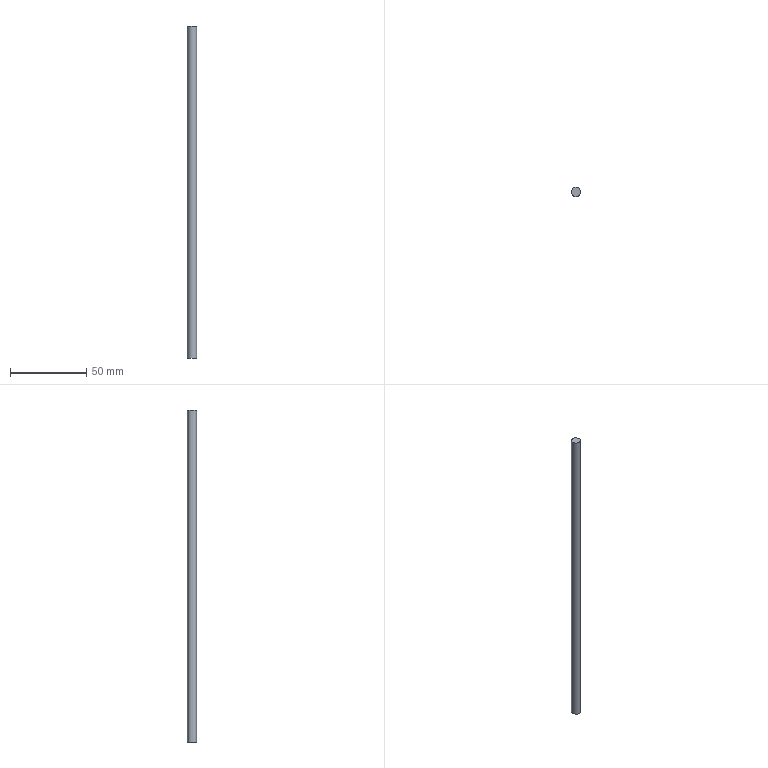Part | NX | features solid 2 | 1 solid | 3 faces | box 6 x 6 x 218 mm | volume 6164 mm3 | plane 2 | cylinder 1 | commonest cylinder face diameters 6 x1
STEP:
#1=CARTESIAN_POINT('',(157.5,-129.5,-423.));
#2=VERTEX_POINT('',#1);
#3=CARTESIAN_POINT('',(157.5,-132.5,-423.));
#4=DIRECTION('',(0.,0.,-1.));
#5=DIRECTION('',(0.,1.,0.));
#6=AXIS2_PLACEMENT_3D('',#3,#4,#5);
#7=CIRCLE('',#6,3.);
#8=EDGE_CURVE('',#2,#2,#7,.T.);
#9=ORIENTED_EDGE('',*,*,#8,.F.);
#10=EDGE_LOOP('',(#9));
#11=FACE_BOUND('',#10,.T.);
#12=CARTESIAN_POINT('',(157.5,-129.5,-205.));
#13=VERTEX_POINT('',#12);
#14=CARTESIAN_POINT('',(157.5,-132.5,-205.));
#15=DIRECTION('',(0.,0.,-1.));
#16=DIRECTION('',(0.,1.,0.));
#17=AXIS2_PLACEMENT_3D('',#14,#15,#16);
#18=CIRCLE('',#17,3.);
#19=EDGE_CURVE('',#13,#13,#18,.T.);
#20=ORIENTED_EDGE('',*,*,#19,.T.);
#21=EDGE_LOOP('',(#20));
#22=FACE_BOUND('',#21,.T.);
#23=CARTESIAN_POINT('',(157.5,-132.5,-423.));
#24=DIRECTION('',(0.,0.,1.));
#25=DIRECTION('',(0.,1.,0.));
#26=AXIS2_PLACEMENT_3D('',#23,#24,#25);
#27=CYLINDRICAL_SURFACE('',#26,3.);
#28=ADVANCED_FACE('',(#11,#22),#27,.T.);
#29=ORIENTED_EDGE('',*,*,#8,.T.);
#30=EDGE_LOOP('',(#29));
#31=FACE_BOUND('',#30,.T.);
#32=CARTESIAN_POINT('',(157.5,-132.5,-423.));
#33=DIRECTION('',(0.,0.,-1.));
#34=DIRECTION('',(0.,-1.,0.));
#35=AXIS2_PLACEMENT_3D('',#32,#33,#34);
#36=PLANE('',#35);
#37=ADVANCED_FACE('',(#31),#36,.T.);
#38=ORIENTED_EDGE('',*,*,#19,.F.);
#39=EDGE_LOOP('',(#38));
#40=FACE_BOUND('',#39,.T.);
#41=CARTESIAN_POINT('',(157.5,-132.5,-205.));
#42=DIRECTION('',(0.,0.,-1.));
#43=DIRECTION('',(0.,-1.,0.));
#44=AXIS2_PLACEMENT_3D('',#41,#42,#43);
#45=PLANE('',#44);
#46=ADVANCED_FACE('',(#40),#45,.F.);
#47=CLOSED_SHELL('',(#28,#37,#46));
#48=MANIFOLD_SOLID_BREP('',#47);
#49=(LENGTH_UNIT()NAMED_UNIT(*)SI_UNIT(.MILLI.,.METRE.));
#50=UNCERTAINTY_MEASURE_WITH_UNIT(LENGTH_MEASURE(0.00001),#49,'','');
#51=(NAMED_UNIT(*)PLANE_ANGLE_UNIT()SI_UNIT($,.RADIAN.));
#52=(NAMED_UNIT(*)SI_UNIT($,.STERADIAN.)SOLID_ANGLE_UNIT());
#53=(GEOMETRIC_REPRESENTATION_CONTEXT(3)GLOBAL_UNCERTAINTY_ASSIGNED_CONTEXT((#50))GLOBAL_UNIT_ASSIGNED_CONTEXT((#49,#51,#52))REPRESENTATION_CONTEXT('',''));
#54=ADVANCED_BREP_SHAPE_REPRESENTATION('',(#48),#53);